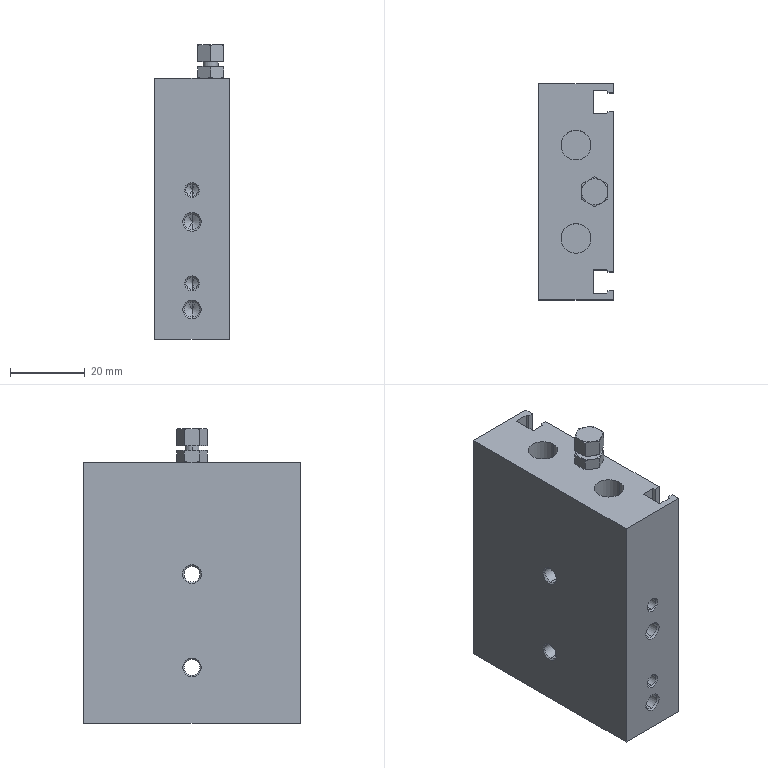Part | SolidWorks | features HoleWzd 10, RefAxis 9, RevCut 4, 3DProfileFeature 3, Revolution 2, Extrusion 1, ICE 1 | 1 solid | 137 faces | box 20 x 58 x 79 mm | volume 67416 mm3 | cone 60 | plane 43 | cylinder 34 | commonest cylinder face diameters 3.242 x8 4.134 x8 8 x8 4.3 x4 15 x4 4 x2